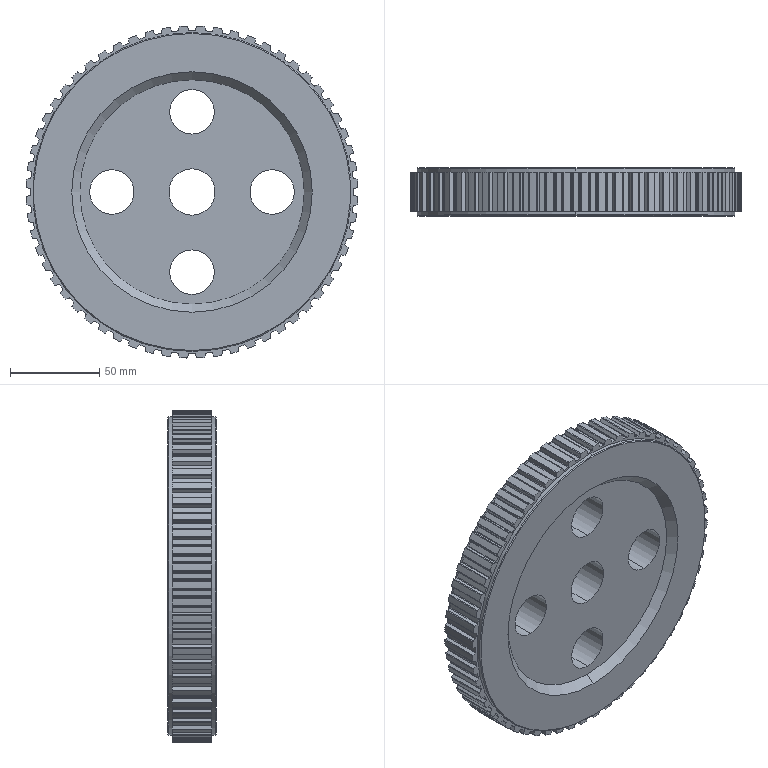Part | SolidWorks | features Cut 5, Chamfer 3, Extrusion 1 | 1 solid | 554 faces | box 186.408 x 27 x 186.408 mm | volume 546884 mm3 | cylinder 360 | plane 186 | cone 8 | commonest cylinder face diameters 0.8 x286 186.5 x60 25 x8 179 x4 26 x2